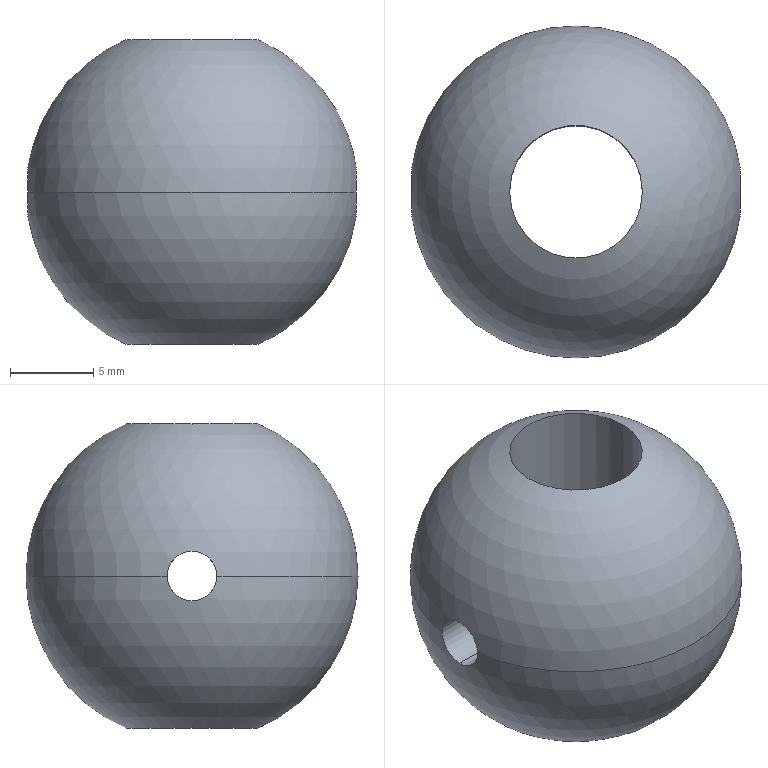Part | SolidWorks | features ICE 2, Revolution 1 | 1 solid | 8 faces | box 19.774 x 20 x 18.33 mm | volume 3140 mm3 | cylinder 6 | sphere 2 | commonest cylinder face diameters 3 x4 8 x2
STEP:
#1=CARTESIAN_POINT('',(4.,0.,1.5));
#2=VERTEX_POINT('',#1);
#3=CARTESIAN_POINT('',(4.,0.,-1.5));
#4=VERTEX_POINT('',#3);
#5=CARTESIAN_POINT('',(4.,0.,1.5));
#6=CARTESIAN_POINT('',(4.,-0.1971,1.5));
#7=CARTESIAN_POINT('',(3.985,-0.396,1.46));
#8=CARTESIAN_POINT('',(3.945,-0.6679,1.347));
#9=CARTESIAN_POINT('',(3.929,-0.7555,1.3));
#10=CARTESIAN_POINT('',(3.894,-0.917,1.191));
#11=CARTESIAN_POINT('',(3.876,-0.9921,1.129));
#12=CARTESIAN_POINT('',(3.818,-1.2,0.9211));
#13=CARTESIAN_POINT('',(3.78,-1.309,0.7577));
#14=CARTESIAN_POINT('',(3.739,-1.423,0.4853));
#15=CARTESIAN_POINT('',(3.727,-1.451,0.3917));
#16=CARTESIAN_POINT('',(3.712,-1.49,0.1987));
#17=CARTESIAN_POINT('',(3.708,-1.5,0.09821));
#18=CARTESIAN_POINT('',(3.708,-1.5,-0.1984));
#19=CARTESIAN_POINT('',(3.725,-1.46,-0.397));
#20=CARTESIAN_POINT('',(3.781,-1.309,-0.7582));
#21=CARTESIAN_POINT('',(3.819,-1.198,-0.9234));
#22=CARTESIAN_POINT('',(3.876,-0.9915,-1.13));
#23=CARTESIAN_POINT('',(3.895,-0.9151,-1.193));
#24=CARTESIAN_POINT('',(3.929,-0.7535,-1.301));
#25=CARTESIAN_POINT('',(3.945,-0.6678,-1.347));
#26=CARTESIAN_POINT('',(3.985,-0.3945,-1.461));
#27=CARTESIAN_POINT('',(4.,-0.2002,-1.5));
#28=CARTESIAN_POINT('',(4.,0.,-1.5));
#29=B_SPLINE_CURVE_WITH_KNOTS('',3,(#5,#6,#7,#8,#9,#10,#11,#12,#13,#14,#15,#16,#17,#18,#19,#20,#21,#22,#23,#24,#25,#26,#27,#28),.UNSPECIFIED.,.F.,.F.,(4,2,2,2,2,2,2,2,2,2,2,4),(0.004733,0.005325,0.005621,0.005916,0.006508,0.006804,0.0071,0.007691,0.008283,0.008578,0.008874,0.009466),.UNSPECIFIED.);
#30=EDGE_CURVE('',#2,#4,#29,.T.);
#31=ORIENTED_EDGE('',*,*,#30,.F.);
#32=CARTESIAN_POINT('',(9.887,0.,1.5));
#33=VERTEX_POINT('',#32);
#34=CARTESIAN_POINT('',(-15.,0.,1.5));
#35=DIRECTION('',(1.,0.,0.));
#36=VECTOR('',#35,1000.);
#37=LINE('',#34,#36);
#38=EDGE_CURVE('',#2,#33,#37,.T.);
#39=ORIENTED_EDGE('',*,*,#38,.T.);
#40=CARTESIAN_POINT('',(9.887,-1.5,0.));
#41=VERTEX_POINT('',#40);
#42=CARTESIAN_POINT('',(9.887,0.,0.));
#43=DIRECTION('',(-1.,0.,0.));
#44=DIRECTION('',(0.,0.,1.));
#45=AXIS2_PLACEMENT_3D('',#42,#43,#44);
#46=CIRCLE('',#45,1.5);
#47=EDGE_CURVE('',#41,#33,#46,.T.);
#48=ORIENTED_EDGE('',*,*,#47,.F.);
#49=CARTESIAN_POINT('',(9.887,0.,-1.5));
#50=VERTEX_POINT('',#49);
#51=CARTESIAN_POINT('',(9.887,0.,0.));
#52=DIRECTION('',(-1.,0.,0.));
#53=DIRECTION('',(0.,0.,1.));
#54=AXIS2_PLACEMENT_3D('',#51,#52,#53);
#55=CIRCLE('',#54,1.5);
#56=EDGE_CURVE('',#50,#41,#55,.T.);
#57=ORIENTED_EDGE('',*,*,#56,.F.);
#58=CARTESIAN_POINT('',(-15.,0.,-1.5));
#59=DIRECTION('',(1.,0.,0.));
#60=VECTOR('',#59,1000.);
#61=LINE('',#58,#60);
#62=EDGE_CURVE('',#4,#50,#61,.T.);
#63=ORIENTED_EDGE('',*,*,#62,.F.);
#64=EDGE_LOOP('',(#31,#39,#48,#57,#63));
#65=FACE_OUTER_BOUND('',#64,.T.);
#66=CARTESIAN_POINT('',(-15.,0.,0.));
#67=DIRECTION('',(1.,0.,0.));
#68=DIRECTION('',(0.,0.,-1.));
#69=AXIS2_PLACEMENT_3D('',#66,#67,#68);
#70=CYLINDRICAL_SURFACE('',#69,1.5);
#71=ADVANCED_FACE('',(#65),#70,.F.);
#72=CARTESIAN_POINT('',(-9.887,0.,1.5));
#73=VERTEX_POINT('',#72);
#74=CARTESIAN_POINT('',(-9.887,-1.5,0.));
#75=VERTEX_POINT('',#74);
#76=CARTESIAN_POINT('',(-9.887,0.,0.));
#77=DIRECTION('',(1.,0.,0.));
#78=DIRECTION('',(0.,0.,-1.));
#79=AXIS2_PLACEMENT_3D('',#76,#77,#78);
#80=CIRCLE('',#79,1.5);
#81=EDGE_CURVE('',#73,#75,#80,.T.);
#82=ORIENTED_EDGE('',*,*,#81,.F.);
#83=CARTESIAN_POINT('',(-4.,0.,1.5));
#84=VERTEX_POINT('',#83);
#85=CARTESIAN_POINT('',(-15.,0.,1.5));
#86=DIRECTION('',(1.,0.,0.));
#87=VECTOR('',#86,1000.);
#88=LINE('',#85,#87);
#89=EDGE_CURVE('',#73,#84,#88,.T.);
#90=ORIENTED_EDGE('',*,*,#89,.T.);
#91=CARTESIAN_POINT('',(-4.,0.,-1.5));
#92=VERTEX_POINT('',#91);
#93=CARTESIAN_POINT('',(-4.,0.,-1.5));
#94=CARTESIAN_POINT('',(-4.,-0.1001,-1.5));
#95=CARTESIAN_POINT('',(-3.996,-0.1983,-1.49));
#96=CARTESIAN_POINT('',(-3.982,-0.3914,-1.451));
#97=CARTESIAN_POINT('',(-3.971,-0.4871,-1.422));
#98=CARTESIAN_POINT('',(-3.932,-0.7591,-1.309));
#99=CARTESIAN_POINT('',(-3.894,-0.9243,-1.197));
#100=CARTESIAN_POINT('',(-3.819,-1.198,-0.923));
#101=CARTESIAN_POINT('',(-3.78,-1.309,-0.7573));
#102=CARTESIAN_POINT('',(-3.739,-1.422,-0.4872));
#103=CARTESIAN_POINT('',(-3.727,-1.451,-0.3917));
#104=CARTESIAN_POINT('',(-3.712,-1.49,-0.1977));
#105=CARTESIAN_POINT('',(-3.708,-1.5,-0.09972));
#106=CARTESIAN_POINT('',(-3.708,-1.5,0.09804));
#107=CARTESIAN_POINT('',(-3.712,-1.49,0.1984));
#108=CARTESIAN_POINT('',(-3.727,-1.451,0.3917));
#109=CARTESIAN_POINT('',(-3.739,-1.423,0.4857));
#110=CARTESIAN_POINT('',(-3.767,-1.346,0.6684));
#111=CARTESIAN_POINT('',(-3.783,-1.3,0.7544));
#112=CARTESIAN_POINT('',(-3.819,-1.192,0.916));
#113=CARTESIAN_POINT('',(-3.838,-1.129,0.9923));
#114=CARTESIAN_POINT('',(-3.876,-0.9914,1.13));
#115=CARTESIAN_POINT('',(-3.894,-0.9166,1.191));
#116=CARTESIAN_POINT('',(-3.929,-0.7545,1.3));
#117=CARTESIAN_POINT('',(-3.945,-0.6669,1.347));
#118=CARTESIAN_POINT('',(-3.984,-0.3963,1.46));
#119=CARTESIAN_POINT('',(-4.,-0.1972,1.5));
#120=CARTESIAN_POINT('',(-4.,0.,1.5));
#121=B_SPLINE_CURVE_WITH_KNOTS('',3,(#93,#94,#95,#96,#97,#98,#99,#100,#101,#102,#103,#104,#105,#106,#107,#108,#109,#110,#111,#112,#113,#114,#115,#116,#117,#118,#119,#120),.UNSPECIFIED.,.F.,.F.,(4,2,2,2,2,2,2,2,2,2,2,2,2,4),(0.,0.0002958,0.0005917,0.001183,0.001775,0.002071,0.002367,0.002663,0.002958,0.003254,0.00355,0.003846,0.004142,0.004733),.UNSPECIFIED.);
#122=EDGE_CURVE('',#92,#84,#121,.T.);
#123=ORIENTED_EDGE('',*,*,#122,.F.);
#124=CARTESIAN_POINT('',(-9.887,0.,-1.5));
#125=VERTEX_POINT('',#124);
#126=CARTESIAN_POINT('',(-15.,0.,-1.5));
#127=DIRECTION('',(1.,0.,0.));
#128=VECTOR('',#127,1000.);
#129=LINE('',#126,#128);
#130=EDGE_CURVE('',#125,#92,#129,.T.);
#131=ORIENTED_EDGE('',*,*,#130,.F.);
#132=CARTESIAN_POINT('',(-9.887,0.,0.));
#133=DIRECTION('',(1.,0.,0.));
#134=DIRECTION('',(0.,0.,-1.));
#135=AXIS2_PLACEMENT_3D('',#132,#133,#134);
#136=CIRCLE('',#135,1.5);
#137=EDGE_CURVE('',#75,#125,#136,.T.);
#138=ORIENTED_EDGE('',*,*,#137,.F.);
#139=EDGE_LOOP('',(#82,#90,#123,#131,#138));
#140=FACE_OUTER_BOUND('',#139,.T.);
#141=CARTESIAN_POINT('',(-15.,0.,0.));
#142=DIRECTION('',(1.,0.,0.));
#143=DIRECTION('',(0.,0.,-1.));
#144=AXIS2_PLACEMENT_3D('',#141,#142,#143);
#145=CYLINDRICAL_SURFACE('',#144,1.5);
#146=ADVANCED_FACE('',(#140),#145,.F.);
#147=CARTESIAN_POINT('',(-4.,0.,-9.165));
#148=VERTEX_POINT('',#147);
#149=CARTESIAN_POINT('',(4.,0.,-9.165));
#150=VERTEX_POINT('',#149);
#151=CARTESIAN_POINT('',(0.,0.,-9.165));
#152=DIRECTION('',(0.,0.,1.));
#153=DIRECTION('',(1.,0.,0.));
#154=AXIS2_PLACEMENT_3D('',#151,#152,#153);
#155=CIRCLE('',#154,4.);
#156=EDGE_CURVE('',#148,#150,#155,.T.);
#157=ORIENTED_EDGE('',*,*,#156,.F.);
#158=CARTESIAN_POINT('',(-4.,0.,-10.));
#159=DIRECTION('',(0.,0.,1.));
#160=VECTOR('',#159,1000.);
#161=LINE('',#158,#160);
#162=EDGE_CURVE('',#148,#92,#161,.T.);
#163=ORIENTED_EDGE('',*,*,#162,.T.);
#164=ORIENTED_EDGE('',*,*,#122,.T.);
#165=CARTESIAN_POINT('',(-4.,0.,9.165));
#166=VERTEX_POINT('',#165);
#167=CARTESIAN_POINT('',(-4.,0.,-10.));
#168=DIRECTION('',(0.,0.,1.));
#169=VECTOR('',#168,1000.);
#170=LINE('',#167,#169);
#171=EDGE_CURVE('',#84,#166,#170,.T.);
#172=ORIENTED_EDGE('',*,*,#171,.T.);
#173=CARTESIAN_POINT('',(4.,0.,9.165));
#174=VERTEX_POINT('',#173);
#175=CARTESIAN_POINT('',(0.,0.,9.165));
#176=DIRECTION('',(0.,0.,-1.));
#177=DIRECTION('',(-1.,0.,0.));
#178=AXIS2_PLACEMENT_3D('',#175,#176,#177);
#179=CIRCLE('',#178,4.);
#180=EDGE_CURVE('',#174,#166,#179,.T.);
#181=ORIENTED_EDGE('',*,*,#180,.F.);
#182=CARTESIAN_POINT('',(4.,0.,-10.));
#183=DIRECTION('',(0.,0.,1.));
#184=VECTOR('',#183,1000.);
#185=LINE('',#182,#184);
#186=EDGE_CURVE('',#2,#174,#185,.T.);
#187=ORIENTED_EDGE('',*,*,#186,.F.);
#188=ORIENTED_EDGE('',*,*,#30,.T.);
#189=CARTESIAN_POINT('',(4.,0.,-10.));
#190=DIRECTION('',(0.,0.,1.));
#191=VECTOR('',#190,1000.);
#192=LINE('',#189,#191);
#193=EDGE_CURVE('',#150,#4,#192,.T.);
#194=ORIENTED_EDGE('',*,*,#193,.F.);
#195=EDGE_LOOP('',(#157,#163,#164,#172,#181,#187,#188,#194));
#196=FACE_OUTER_BOUND('',#195,.T.);
#197=CARTESIAN_POINT('',(0.,0.,-10.));
#198=DIRECTION('',(0.,0.,1.));
#199=DIRECTION('',(1.,0.,0.));
#200=AXIS2_PLACEMENT_3D('',#197,#198,#199);
#201=CYLINDRICAL_SURFACE('',#200,4.);
#202=ADVANCED_FACE('',(#196),#201,.F.);
#203=CARTESIAN_POINT('',(0.,0.,-9.165));
#204=DIRECTION('',(0.,0.,1.));
#205=DIRECTION('',(1.,0.,0.));
#206=AXIS2_PLACEMENT_3D('',#203,#204,#205);
#207=CIRCLE('',#206,4.);
#208=EDGE_CURVE('',#150,#148,#207,.T.);
#209=ORIENTED_EDGE('',*,*,#208,.T.);
#210=ORIENTED_EDGE('',*,*,#156,.T.);
#211=EDGE_LOOP('',(#209,#210));
#212=FACE_BOUND('',#211,.T.);
#213=CARTESIAN_POINT('',(0.,-10.,0.));
#214=VERTEX_POINT('',#213);
#215=CARTESIAN_POINT('',(0.,0.,0.));
#216=DIRECTION('',(0.,0.,1.));
#217=DIRECTION('',(1.,0.,0.));
#218=AXIS2_PLACEMENT_3D('',#215,#216,#217);
#219=CIRCLE('',#218,10.);
#220=EDGE_CURVE('',#214,#41,#219,.T.);
#221=ORIENTED_EDGE('',*,*,#220,.F.);
#222=CARTESIAN_POINT('',(0.,0.,0.));
#223=DIRECTION('',(0.,0.,-1.));
#224=DIRECTION('',(-1.,0.,0.));
#225=AXIS2_PLACEMENT_3D('',#222,#223,#224);
#226=CIRCLE('',#225,10.);
#227=EDGE_CURVE('',#214,#75,#226,.T.);
#228=ORIENTED_EDGE('',*,*,#227,.T.);
#229=ORIENTED_EDGE('',*,*,#137,.T.);
#230=CARTESIAN_POINT('',(-9.887,1.5,0.));
#231=VERTEX_POINT('',#230);
#232=CARTESIAN_POINT('',(-9.887,0.,0.));
#233=DIRECTION('',(1.,0.,0.));
#234=DIRECTION('',(0.,0.,-1.));
#235=AXIS2_PLACEMENT_3D('',#232,#233,#234);
#236=CIRCLE('',#235,1.5);
#237=EDGE_CURVE('',#125,#231,#236,.T.);
#238=ORIENTED_EDGE('',*,*,#237,.T.);
#239=CARTESIAN_POINT('',(0.,10.,0.));
#240=VERTEX_POINT('',#239);
#241=CARTESIAN_POINT('',(0.,0.,0.));
#242=DIRECTION('',(0.,0.,-1.));
#243=DIRECTION('',(-1.,0.,0.));
#244=AXIS2_PLACEMENT_3D('',#241,#242,#243);
#245=CIRCLE('',#244,10.);
#246=EDGE_CURVE('',#231,#240,#245,.T.);
#247=ORIENTED_EDGE('',*,*,#246,.T.);
#248=CARTESIAN_POINT('',(9.887,1.5,0.));
#249=VERTEX_POINT('',#248);
#250=CARTESIAN_POINT('',(0.,0.,0.));
#251=DIRECTION('',(0.,0.,1.));
#252=DIRECTION('',(1.,0.,0.));
#253=AXIS2_PLACEMENT_3D('',#250,#251,#252);
#254=CIRCLE('',#253,10.);
#255=EDGE_CURVE('',#249,#240,#254,.T.);
#256=ORIENTED_EDGE('',*,*,#255,.F.);
#257=CARTESIAN_POINT('',(9.887,0.,0.));
#258=DIRECTION('',(-1.,0.,0.));
#259=DIRECTION('',(0.,0.,1.));
#260=AXIS2_PLACEMENT_3D('',#257,#258,#259);
#261=CIRCLE('',#260,1.5);
#262=EDGE_CURVE('',#249,#50,#261,.T.);
#263=ORIENTED_EDGE('',*,*,#262,.T.);
#264=ORIENTED_EDGE('',*,*,#56,.T.);
#265=EDGE_LOOP('',(#221,#228,#229,#238,#247,#256,#263,#264));
#266=FACE_OUTER_BOUND('',#265,.T.);
#267=CARTESIAN_POINT('',(0.,0.,0.));
#268=DIRECTION('',(0.,0.,-1.));
#269=DIRECTION('',(1.,0.,0.));
#270=AXIS2_PLACEMENT_3D('',#267,#268,#269);
#271=SPHERICAL_SURFACE('',#270,10.);
#272=ADVANCED_FACE('',(#212,#266),#271,.T.);
#273=ORIENTED_EDGE('',*,*,#227,.F.);
#274=ORIENTED_EDGE('',*,*,#220,.T.);
#275=ORIENTED_EDGE('',*,*,#47,.T.);
#276=CARTESIAN_POINT('',(9.887,0.,0.));
#277=DIRECTION('',(-1.,0.,0.));
#278=DIRECTION('',(0.,0.,1.));
#279=AXIS2_PLACEMENT_3D('',#276,#277,#278);
#280=CIRCLE('',#279,1.5);
#281=EDGE_CURVE('',#33,#249,#280,.T.);
#282=ORIENTED_EDGE('',*,*,#281,.T.);
#283=ORIENTED_EDGE('',*,*,#255,.T.);
#284=ORIENTED_EDGE('',*,*,#246,.F.);
#285=CARTESIAN_POINT('',(-9.887,0.,0.));
#286=DIRECTION('',(1.,0.,0.));
#287=DIRECTION('',(0.,0.,-1.));
#288=AXIS2_PLACEMENT_3D('',#285,#286,#287);
#289=CIRCLE('',#288,1.5);
#290=EDGE_CURVE('',#231,#73,#289,.T.);
#291=ORIENTED_EDGE('',*,*,#290,.T.);
#292=ORIENTED_EDGE('',*,*,#81,.T.);
#293=EDGE_LOOP('',(#273,#274,#275,#282,#283,#284,#291,#292));
#294=FACE_OUTER_BOUND('',#293,.T.);
#295=ORIENTED_EDGE('',*,*,#180,.T.);
#296=CARTESIAN_POINT('',(0.,0.,9.165));
#297=DIRECTION('',(0.,0.,-1.));
#298=DIRECTION('',(-1.,0.,0.));
#299=AXIS2_PLACEMENT_3D('',#296,#297,#298);
#300=CIRCLE('',#299,4.);
#301=EDGE_CURVE('',#166,#174,#300,.T.);
#302=ORIENTED_EDGE('',*,*,#301,.T.);
#303=EDGE_LOOP('',(#295,#302));
#304=FACE_BOUND('',#303,.T.);
#305=CARTESIAN_POINT('',(0.,0.,0.));
#306=DIRECTION('',(0.,0.,-1.));
#307=DIRECTION('',(1.,0.,0.));
#308=AXIS2_PLACEMENT_3D('',#305,#306,#307);
#309=SPHERICAL_SURFACE('',#308,10.);
#310=ADVANCED_FACE('',(#294,#304),#309,.T.);
#311=ORIENTED_EDGE('',*,*,#162,.F.);
#312=ORIENTED_EDGE('',*,*,#208,.F.);
#313=ORIENTED_EDGE('',*,*,#193,.T.);
#314=CARTESIAN_POINT('',(4.,0.,-1.5));
#315=CARTESIAN_POINT('',(4.,0.1001,-1.5));
#316=CARTESIAN_POINT('',(3.996,0.1983,-1.49));
#317=CARTESIAN_POINT('',(3.982,0.3914,-1.451));
#318=CARTESIAN_POINT('',(3.971,0.4871,-1.422));
#319=CARTESIAN_POINT('',(3.932,0.7591,-1.309));
#320=CARTESIAN_POINT('',(3.894,0.9243,-1.197));
#321=CARTESIAN_POINT('',(3.819,1.198,-0.923));
#322=CARTESIAN_POINT('',(3.78,1.309,-0.7573));
#323=CARTESIAN_POINT('',(3.739,1.422,-0.4872));
#324=CARTESIAN_POINT('',(3.727,1.451,-0.3917));
#325=CARTESIAN_POINT('',(3.712,1.49,-0.1977));
#326=CARTESIAN_POINT('',(3.708,1.5,-0.09972));
#327=CARTESIAN_POINT('',(3.708,1.5,0.09804));
#328=CARTESIAN_POINT('',(3.712,1.49,0.1984));
#329=CARTESIAN_POINT('',(3.727,1.451,0.3917));
#330=CARTESIAN_POINT('',(3.739,1.423,0.4857));
#331=CARTESIAN_POINT('',(3.767,1.346,0.6684));
#332=CARTESIAN_POINT('',(3.783,1.3,0.7544));
#333=CARTESIAN_POINT('',(3.819,1.192,0.916));
#334=CARTESIAN_POINT('',(3.838,1.129,0.9923));
#335=CARTESIAN_POINT('',(3.876,0.9914,1.13));
#336=CARTESIAN_POINT('',(3.894,0.9166,1.191));
#337=CARTESIAN_POINT('',(3.929,0.7545,1.3));
#338=CARTESIAN_POINT('',(3.945,0.6669,1.347));
#339=CARTESIAN_POINT('',(3.984,0.3963,1.46));
#340=CARTESIAN_POINT('',(4.,0.1972,1.5));
#341=CARTESIAN_POINT('',(4.,0.,1.5));
#342=B_SPLINE_CURVE_WITH_KNOTS('',3,(#314,#315,#316,#317,#318,#319,#320,#321,#322,#323,#324,#325,#326,#327,#328,#329,#330,#331,#332,#333,#334,#335,#336,#337,#338,#339,#340,#341),.UNSPECIFIED.,.F.,.F.,(4,2,2,2,2,2,2,2,2,2,2,2,2,4),(0.,0.0002958,0.0005917,0.001183,0.001775,0.002071,0.002367,0.002663,0.002958,0.003254,0.00355,0.003846,0.004142,0.004733),.UNSPECIFIED.);
#343=EDGE_CURVE('',#4,#2,#342,.T.);
#344=ORIENTED_EDGE('',*,*,#343,.T.);
#345=ORIENTED_EDGE('',*,*,#186,.T.);
#346=ORIENTED_EDGE('',*,*,#301,.F.);
#347=ORIENTED_EDGE('',*,*,#171,.F.);
#348=CARTESIAN_POINT('',(-4.,0.,1.5));
#349=CARTESIAN_POINT('',(-4.,0.1971,1.5));
#350=CARTESIAN_POINT('',(-3.985,0.396,1.46));
#351=CARTESIAN_POINT('',(-3.945,0.6679,1.347));
#352=CARTESIAN_POINT('',(-3.929,0.7555,1.3));
#353=CARTESIAN_POINT('',(-3.894,0.917,1.191));
#354=CARTESIAN_POINT('',(-3.876,0.9921,1.129));
#355=CARTESIAN_POINT('',(-3.818,1.2,0.9211));
#356=CARTESIAN_POINT('',(-3.78,1.309,0.7577));
#357=CARTESIAN_POINT('',(-3.739,1.423,0.4853));
#358=CARTESIAN_POINT('',(-3.727,1.451,0.3917));
#359=CARTESIAN_POINT('',(-3.712,1.49,0.1987));
#360=CARTESIAN_POINT('',(-3.708,1.5,0.09821));
#361=CARTESIAN_POINT('',(-3.708,1.5,-0.1984));
#362=CARTESIAN_POINT('',(-3.725,1.46,-0.397));
#363=CARTESIAN_POINT('',(-3.781,1.309,-0.7582));
#364=CARTESIAN_POINT('',(-3.819,1.198,-0.9234));
#365=CARTESIAN_POINT('',(-3.876,0.9915,-1.13));
#366=CARTESIAN_POINT('',(-3.895,0.9151,-1.193));
#367=CARTESIAN_POINT('',(-3.929,0.7535,-1.301));
#368=CARTESIAN_POINT('',(-3.945,0.6678,-1.347));
#369=CARTESIAN_POINT('',(-3.985,0.3945,-1.461));
#370=CARTESIAN_POINT('',(-4.,0.2002,-1.5));
#371=CARTESIAN_POINT('',(-4.,0.,-1.5));
#372=B_SPLINE_CURVE_WITH_KNOTS('',3,(#348,#349,#350,#351,#352,#353,#354,#355,#356,#357,#358,#359,#360,#361,#362,#363,#364,#365,#366,#367,#368,#369,#370,#371),.UNSPECIFIED.,.F.,.F.,(4,2,2,2,2,2,2,2,2,2,2,4),(0.004733,0.005325,0.005621,0.005916,0.006508,0.006804,0.0071,0.007691,0.008283,0.008578,0.008874,0.009466),.UNSPECIFIED.);
#373=EDGE_CURVE('',#84,#92,#372,.T.);
#374=ORIENTED_EDGE('',*,*,#373,.T.);
#375=EDGE_LOOP('',(#311,#312,#313,#344,#345,#346,#347,#374));
#376=FACE_OUTER_BOUND('',#375,.T.);
#377=CARTESIAN_POINT('',(0.,0.,-10.));
#378=DIRECTION('',(0.,0.,1.));
#379=DIRECTION('',(1.,0.,0.));
#380=AXIS2_PLACEMENT_3D('',#377,#378,#379);
#381=CYLINDRICAL_SURFACE('',#380,4.);
#382=ADVANCED_FACE('',(#376),#381,.F.);
#383=ORIENTED_EDGE('',*,*,#89,.F.);
#384=ORIENTED_EDGE('',*,*,#290,.F.);
#385=ORIENTED_EDGE('',*,*,#237,.F.);
#386=ORIENTED_EDGE('',*,*,#130,.T.);
#387=ORIENTED_EDGE('',*,*,#373,.F.);
#388=EDGE_LOOP('',(#383,#384,#385,#386,#387));
#389=FACE_OUTER_BOUND('',#388,.T.);
#390=CARTESIAN_POINT('',(-15.,0.,0.));
#391=DIRECTION('',(1.,0.,0.));
#392=DIRECTION('',(0.,0.,-1.));
#393=AXIS2_PLACEMENT_3D('',#390,#391,#392);
#394=CYLINDRICAL_SURFACE('',#393,1.5);
#395=ADVANCED_FACE('',(#389),#394,.F.);
#396=ORIENTED_EDGE('',*,*,#38,.F.);
#397=ORIENTED_EDGE('',*,*,#343,.F.);
#398=ORIENTED_EDGE('',*,*,#62,.T.);
#399=ORIENTED_EDGE('',*,*,#262,.F.);
#400=ORIENTED_EDGE('',*,*,#281,.F.);
#401=EDGE_LOOP('',(#396,#397,#398,#399,#400));
#402=FACE_OUTER_BOUND('',#401,.T.);
#403=CARTESIAN_POINT('',(-15.,0.,0.));
#404=DIRECTION('',(1.,0.,0.));
#405=DIRECTION('',(0.,0.,-1.));
#406=AXIS2_PLACEMENT_3D('',#403,#404,#405);
#407=CYLINDRICAL_SURFACE('',#406,1.5);
#408=ADVANCED_FACE('',(#402),#407,.F.);
#409=CLOSED_SHELL('',(#71,#146,#202,#272,#310,#382,#395,#408));
#410=MANIFOLD_SOLID_BREP('',#409);
#411=CARTESIAN_POINT('',(0.,0.,0.));
#412=DIRECTION('',(0.,0.,1.));
#413=DIRECTION('',(1.,0.,0.));
#414=AXIS2_PLACEMENT_3D('',#411,#412,#413);
#415=(LENGTH_UNIT()NAMED_UNIT(*)SI_UNIT(.MILLI.,.METRE.));
#416=UNCERTAINTY_MEASURE_WITH_UNIT(LENGTH_MEASURE(0.00001),#415,'','');
#417=(NAMED_UNIT(*)PLANE_ANGLE_UNIT()SI_UNIT($,.RADIAN.));
#418=(NAMED_UNIT(*)SI_UNIT($,.STERADIAN.)SOLID_ANGLE_UNIT());
#419=(GEOMETRIC_REPRESENTATION_CONTEXT(3)GLOBAL_UNCERTAINTY_ASSIGNED_CONTEXT((#416))GLOBAL_UNIT_ASSIGNED_CONTEXT((#415,#417,#418))REPRESENTATION_CONTEXT('',''));
#420=ADVANCED_BREP_SHAPE_REPRESENTATION('',(#410,#414),#419);